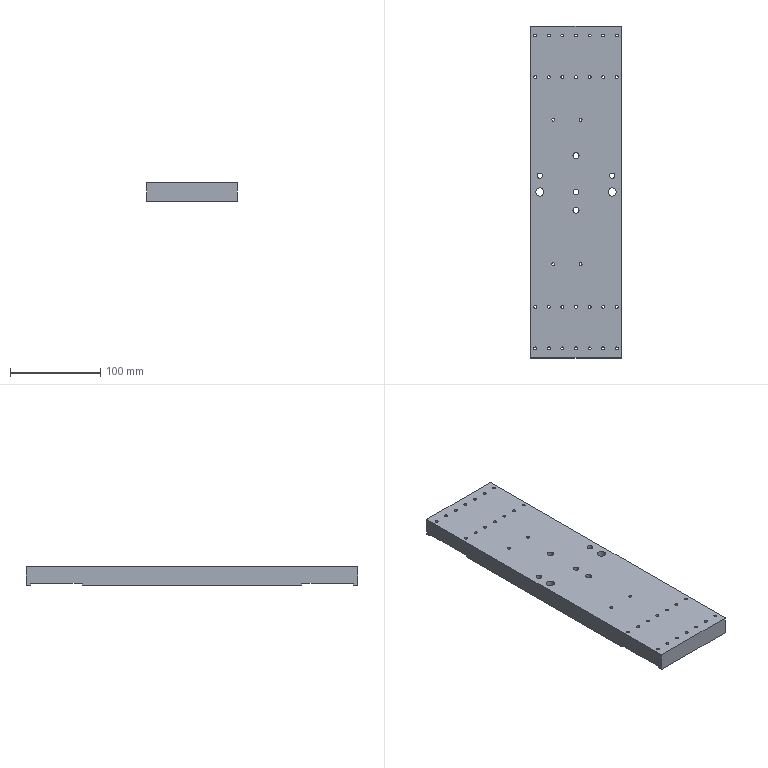Part | 1 solid | 53 faces | box 100 x 367 x 20 mm | volume 700511 mm3 | cylinder 39 | plane 14 | commonest cylinder face diameters 3.3 x32 6 x3 6.8 x2 9 x2